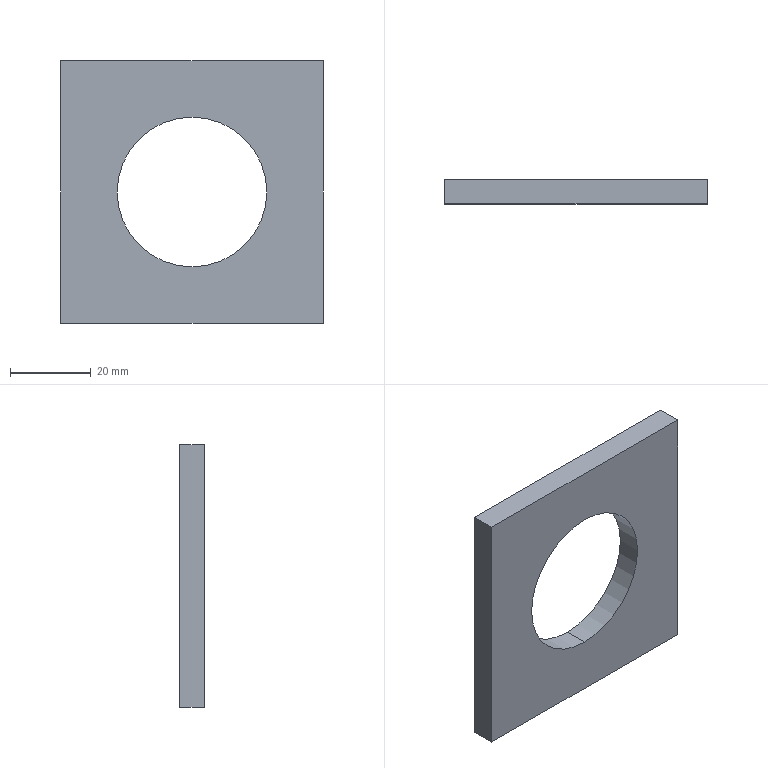Part | SolidWorks | features Extrusion 1 | 1 solid | 8 faces | box 65 x 6 x 65 mm | volume 18899 mm3 | plane 6 | cylinder 2 | commonest cylinder face diameters 37 x2
STEP:
#1=CARTESIAN_POINT('',(0.,3.,-18.5));
#2=VERTEX_POINT('',#1);
#3=CARTESIAN_POINT('',(0.,3.,18.5));
#4=VERTEX_POINT('',#3);
#5=CARTESIAN_POINT('',(0.,3.,0.));
#6=DIRECTION('',(0.,1.,0.));
#7=DIRECTION('',(0.,0.,1.));
#8=AXIS2_PLACEMENT_3D('',#5,#6,#7);
#9=CIRCLE('',#8,18.5);
#10=EDGE_CURVE('',#2,#4,#9,.T.);
#11=ORIENTED_EDGE('',*,*,#10,.T.);
#12=CARTESIAN_POINT('',(0.,-3.,18.5));
#13=VERTEX_POINT('',#12);
#14=CARTESIAN_POINT('',(0.,3.,18.5));
#15=DIRECTION('',(0.,-1.,0.));
#16=VECTOR('',#15,1000.);
#17=LINE('',#14,#16);
#18=EDGE_CURVE('',#4,#13,#17,.T.);
#19=ORIENTED_EDGE('',*,*,#18,.T.);
#20=CARTESIAN_POINT('',(0.,-3.,-18.5));
#21=VERTEX_POINT('',#20);
#22=CARTESIAN_POINT('',(0.,-3.,0.));
#23=DIRECTION('',(0.,1.,0.));
#24=DIRECTION('',(0.,0.,1.));
#25=AXIS2_PLACEMENT_3D('',#22,#23,#24);
#26=CIRCLE('',#25,18.5);
#27=EDGE_CURVE('',#21,#13,#26,.T.);
#28=ORIENTED_EDGE('',*,*,#27,.F.);
#29=CARTESIAN_POINT('',(0.,3.,-18.5));
#30=DIRECTION('',(0.,-1.,0.));
#31=VECTOR('',#30,1000.);
#32=LINE('',#29,#31);
#33=EDGE_CURVE('',#2,#21,#32,.T.);
#34=ORIENTED_EDGE('',*,*,#33,.F.);
#35=EDGE_LOOP('',(#11,#19,#28,#34));
#36=FACE_OUTER_BOUND('',#35,.T.);
#37=CARTESIAN_POINT('',(0.,3.,0.));
#38=DIRECTION('',(0.,-1.,0.));
#39=DIRECTION('',(0.,0.,-1.));
#40=AXIS2_PLACEMENT_3D('',#37,#38,#39);
#41=CYLINDRICAL_SURFACE('',#40,18.5);
#42=ADVANCED_FACE('',(#36),#41,.F.);
#43=CARTESIAN_POINT('',(-32.5,3.,-32.5));
#44=VERTEX_POINT('',#43);
#45=CARTESIAN_POINT('',(-32.5,3.,32.5));
#46=VERTEX_POINT('',#45);
#47=CARTESIAN_POINT('',(-32.5,3.,-32.5));
#48=DIRECTION('',(0.,0.,1.));
#49=VECTOR('',#48,1000.);
#50=LINE('',#47,#49);
#51=EDGE_CURVE('',#44,#46,#50,.T.);
#52=ORIENTED_EDGE('',*,*,#51,.T.);
#53=CARTESIAN_POINT('',(32.5,3.,32.5));
#54=VERTEX_POINT('',#53);
#55=CARTESIAN_POINT('',(-32.5,3.,32.5));
#56=DIRECTION('',(1.,0.,0.));
#57=VECTOR('',#56,1000.);
#58=LINE('',#55,#57);
#59=EDGE_CURVE('',#46,#54,#58,.T.);
#60=ORIENTED_EDGE('',*,*,#59,.T.);
#61=CARTESIAN_POINT('',(32.5,3.,-32.5));
#62=VERTEX_POINT('',#61);
#63=CARTESIAN_POINT('',(32.5,3.,-32.5));
#64=DIRECTION('',(0.,0.,-1.));
#65=VECTOR('',#64,1000.);
#66=LINE('',#63,#65);
#67=EDGE_CURVE('',#54,#62,#66,.T.);
#68=ORIENTED_EDGE('',*,*,#67,.T.);
#69=CARTESIAN_POINT('',(-32.5,3.,-32.5));
#70=DIRECTION('',(-1.,0.,0.));
#71=VECTOR('',#70,1000.);
#72=LINE('',#69,#71);
#73=EDGE_CURVE('',#62,#44,#72,.T.);
#74=ORIENTED_EDGE('',*,*,#73,.T.);
#75=EDGE_LOOP('',(#52,#60,#68,#74));
#76=FACE_OUTER_BOUND('',#75,.T.);
#77=ORIENTED_EDGE('',*,*,#10,.F.);
#78=CARTESIAN_POINT('',(0.,3.,0.));
#79=DIRECTION('',(0.,1.,0.));
#80=DIRECTION('',(0.,0.,1.));
#81=AXIS2_PLACEMENT_3D('',#78,#79,#80);
#82=CIRCLE('',#81,18.5);
#83=EDGE_CURVE('',#4,#2,#82,.T.);
#84=ORIENTED_EDGE('',*,*,#83,.F.);
#85=EDGE_LOOP('',(#77,#84));
#86=FACE_BOUND('',#85,.T.);
#87=CARTESIAN_POINT('',(-32.5,3.,32.5));
#88=DIRECTION('',(0.,1.,0.));
#89=DIRECTION('',(0.,0.,1.));
#90=AXIS2_PLACEMENT_3D('',#87,#88,#89);
#91=PLANE('',#90);
#92=ADVANCED_FACE('',(#76,#86),#91,.T.);
#93=CARTESIAN_POINT('',(-32.5,-3.,-32.5));
#94=VERTEX_POINT('',#93);
#95=CARTESIAN_POINT('',(-32.5,-3.,32.5));
#96=VERTEX_POINT('',#95);
#97=CARTESIAN_POINT('',(-32.5,-3.,-32.5));
#98=DIRECTION('',(0.,0.,1.));
#99=VECTOR('',#98,1000.);
#100=LINE('',#97,#99);
#101=EDGE_CURVE('',#94,#96,#100,.T.);
#102=ORIENTED_EDGE('',*,*,#101,.F.);
#103=CARTESIAN_POINT('',(32.5,-3.,-32.5));
#104=VERTEX_POINT('',#103);
#105=CARTESIAN_POINT('',(-32.5,-3.,-32.5));
#106=DIRECTION('',(-1.,0.,0.));
#107=VECTOR('',#106,1000.);
#108=LINE('',#105,#107);
#109=EDGE_CURVE('',#104,#94,#108,.T.);
#110=ORIENTED_EDGE('',*,*,#109,.F.);
#111=CARTESIAN_POINT('',(32.5,-3.,32.5));
#112=VERTEX_POINT('',#111);
#113=CARTESIAN_POINT('',(32.5,-3.,-32.5));
#114=DIRECTION('',(0.,0.,-1.));
#115=VECTOR('',#114,1000.);
#116=LINE('',#113,#115);
#117=EDGE_CURVE('',#112,#104,#116,.T.);
#118=ORIENTED_EDGE('',*,*,#117,.F.);
#119=CARTESIAN_POINT('',(-32.5,-3.,32.5));
#120=DIRECTION('',(1.,0.,0.));
#121=VECTOR('',#120,1000.);
#122=LINE('',#119,#121);
#123=EDGE_CURVE('',#96,#112,#122,.T.);
#124=ORIENTED_EDGE('',*,*,#123,.F.);
#125=EDGE_LOOP('',(#102,#110,#118,#124));
#126=FACE_OUTER_BOUND('',#125,.T.);
#127=ORIENTED_EDGE('',*,*,#27,.T.);
#128=CARTESIAN_POINT('',(0.,-3.,0.));
#129=DIRECTION('',(0.,1.,0.));
#130=DIRECTION('',(0.,0.,1.));
#131=AXIS2_PLACEMENT_3D('',#128,#129,#130);
#132=CIRCLE('',#131,18.5);
#133=EDGE_CURVE('',#13,#21,#132,.T.);
#134=ORIENTED_EDGE('',*,*,#133,.T.);
#135=EDGE_LOOP('',(#127,#134));
#136=FACE_BOUND('',#135,.T.);
#137=CARTESIAN_POINT('',(-32.5,-3.,32.5));
#138=DIRECTION('',(0.,1.,0.));
#139=DIRECTION('',(0.,0.,1.));
#140=AXIS2_PLACEMENT_3D('',#137,#138,#139);
#141=PLANE('',#140);
#142=ADVANCED_FACE('',(#126,#136),#141,.F.);
#143=ORIENTED_EDGE('',*,*,#101,.T.);
#144=CARTESIAN_POINT('',(-32.5,3.,32.5));
#145=DIRECTION('',(0.,-1.,0.));
#146=VECTOR('',#145,1000.);
#147=LINE('',#144,#146);
#148=EDGE_CURVE('',#46,#96,#147,.T.);
#149=ORIENTED_EDGE('',*,*,#148,.F.);
#150=ORIENTED_EDGE('',*,*,#51,.F.);
#151=CARTESIAN_POINT('',(-32.5,3.,-32.5));
#152=DIRECTION('',(0.,-1.,0.));
#153=VECTOR('',#152,1000.);
#154=LINE('',#151,#153);
#155=EDGE_CURVE('',#44,#94,#154,.T.);
#156=ORIENTED_EDGE('',*,*,#155,.T.);
#157=EDGE_LOOP('',(#143,#149,#150,#156));
#158=FACE_OUTER_BOUND('',#157,.T.);
#159=CARTESIAN_POINT('',(-32.5,3.,-32.5));
#160=DIRECTION('',(1.,0.,0.));
#161=DIRECTION('',(0.,0.,-1.));
#162=AXIS2_PLACEMENT_3D('',#159,#160,#161);
#163=PLANE('',#162);
#164=ADVANCED_FACE('',(#158),#163,.F.);
#165=ORIENTED_EDGE('',*,*,#123,.T.);
#166=CARTESIAN_POINT('',(32.5,3.,32.5));
#167=DIRECTION('',(0.,-1.,0.));
#168=VECTOR('',#167,1000.);
#169=LINE('',#166,#168);
#170=EDGE_CURVE('',#54,#112,#169,.T.);
#171=ORIENTED_EDGE('',*,*,#170,.F.);
#172=ORIENTED_EDGE('',*,*,#59,.F.);
#173=ORIENTED_EDGE('',*,*,#148,.T.);
#174=EDGE_LOOP('',(#165,#171,#172,#173));
#175=FACE_OUTER_BOUND('',#174,.T.);
#176=CARTESIAN_POINT('',(-32.5,3.,32.5));
#177=DIRECTION('',(0.,0.,-1.));
#178=DIRECTION('',(-1.,0.,0.));
#179=AXIS2_PLACEMENT_3D('',#176,#177,#178);
#180=PLANE('',#179);
#181=ADVANCED_FACE('',(#175),#180,.F.);
#182=ORIENTED_EDGE('',*,*,#117,.T.);
#183=CARTESIAN_POINT('',(32.5,3.,-32.5));
#184=DIRECTION('',(0.,-1.,0.));
#185=VECTOR('',#184,1000.);
#186=LINE('',#183,#185);
#187=EDGE_CURVE('',#62,#104,#186,.T.);
#188=ORIENTED_EDGE('',*,*,#187,.F.);
#189=ORIENTED_EDGE('',*,*,#67,.F.);
#190=ORIENTED_EDGE('',*,*,#170,.T.);
#191=EDGE_LOOP('',(#182,#188,#189,#190));
#192=FACE_OUTER_BOUND('',#191,.T.);
#193=CARTESIAN_POINT('',(32.5,3.,-32.5));
#194=DIRECTION('',(-1.,0.,0.));
#195=DIRECTION('',(0.,0.,1.));
#196=AXIS2_PLACEMENT_3D('',#193,#194,#195);
#197=PLANE('',#196);
#198=ADVANCED_FACE('',(#192),#197,.F.);
#199=ORIENTED_EDGE('',*,*,#109,.T.);
#200=ORIENTED_EDGE('',*,*,#155,.F.);
#201=ORIENTED_EDGE('',*,*,#73,.F.);
#202=ORIENTED_EDGE('',*,*,#187,.T.);
#203=EDGE_LOOP('',(#199,#200,#201,#202));
#204=FACE_OUTER_BOUND('',#203,.T.);
#205=CARTESIAN_POINT('',(-32.5,3.,-32.5));
#206=DIRECTION('',(0.,0.,1.));
#207=DIRECTION('',(1.,0.,0.));
#208=AXIS2_PLACEMENT_3D('',#205,#206,#207);
#209=PLANE('',#208);
#210=ADVANCED_FACE('',(#204),#209,.F.);
#211=ORIENTED_EDGE('',*,*,#18,.F.);
#212=ORIENTED_EDGE('',*,*,#83,.T.);
#213=ORIENTED_EDGE('',*,*,#33,.T.);
#214=ORIENTED_EDGE('',*,*,#133,.F.);
#215=EDGE_LOOP('',(#211,#212,#213,#214));
#216=FACE_OUTER_BOUND('',#215,.T.);
#217=CARTESIAN_POINT('',(0.,3.,0.));
#218=DIRECTION('',(0.,-1.,0.));
#219=DIRECTION('',(0.,0.,-1.));
#220=AXIS2_PLACEMENT_3D('',#217,#218,#219);
#221=CYLINDRICAL_SURFACE('',#220,18.5);
#222=ADVANCED_FACE('',(#216),#221,.F.);
#223=CLOSED_SHELL('',(#42,#92,#142,#164,#181,#198,#210,#222));
#224=MANIFOLD_SOLID_BREP('',#223);
#225=CARTESIAN_POINT('',(0.,0.,0.));
#226=DIRECTION('',(0.,0.,1.));
#227=DIRECTION('',(1.,0.,0.));
#228=AXIS2_PLACEMENT_3D('',#225,#226,#227);
#229=(LENGTH_UNIT()NAMED_UNIT(*)SI_UNIT(.MILLI.,.METRE.));
#230=UNCERTAINTY_MEASURE_WITH_UNIT(LENGTH_MEASURE(0.00001),#229,'','');
#231=(NAMED_UNIT(*)PLANE_ANGLE_UNIT()SI_UNIT($,.RADIAN.));
#232=(NAMED_UNIT(*)SI_UNIT($,.STERADIAN.)SOLID_ANGLE_UNIT());
#233=(GEOMETRIC_REPRESENTATION_CONTEXT(3)GLOBAL_UNCERTAINTY_ASSIGNED_CONTEXT((#230))GLOBAL_UNIT_ASSIGNED_CONTEXT((#229,#231,#232))REPRESENTATION_CONTEXT('',''));
#234=ADVANCED_BREP_SHAPE_REPRESENTATION('',(#224,#228),#233);